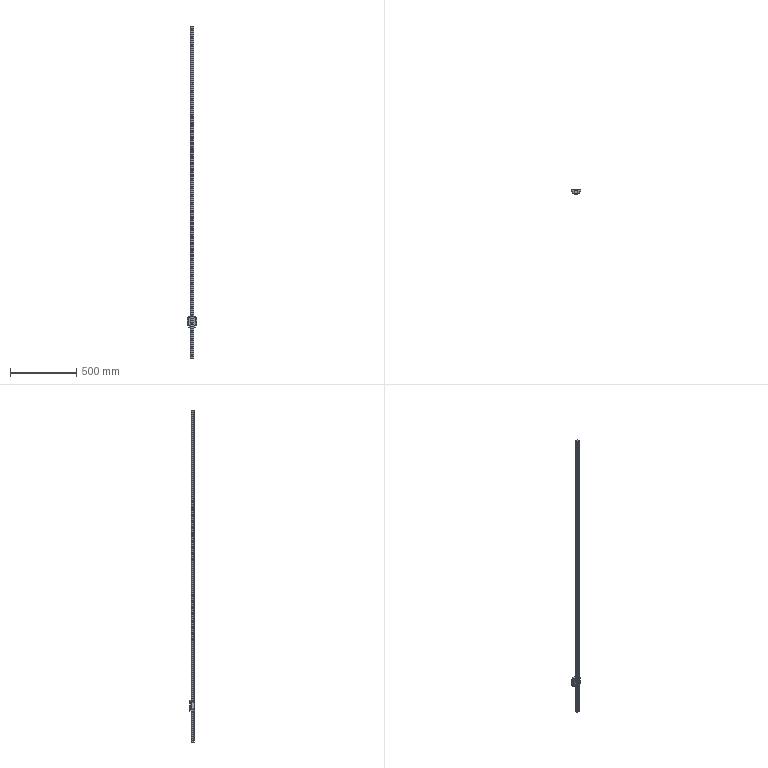Part | SolidWorks | 2 solids | 334 faces | box 70 x 36 x 2500 mm | volume 1159960 mm3 | cylinder 192 | plane 142 | commonest cylinder face diameters 11 x88 6.6 x78 4.6 x8 8 x8 7 x6 3 x4